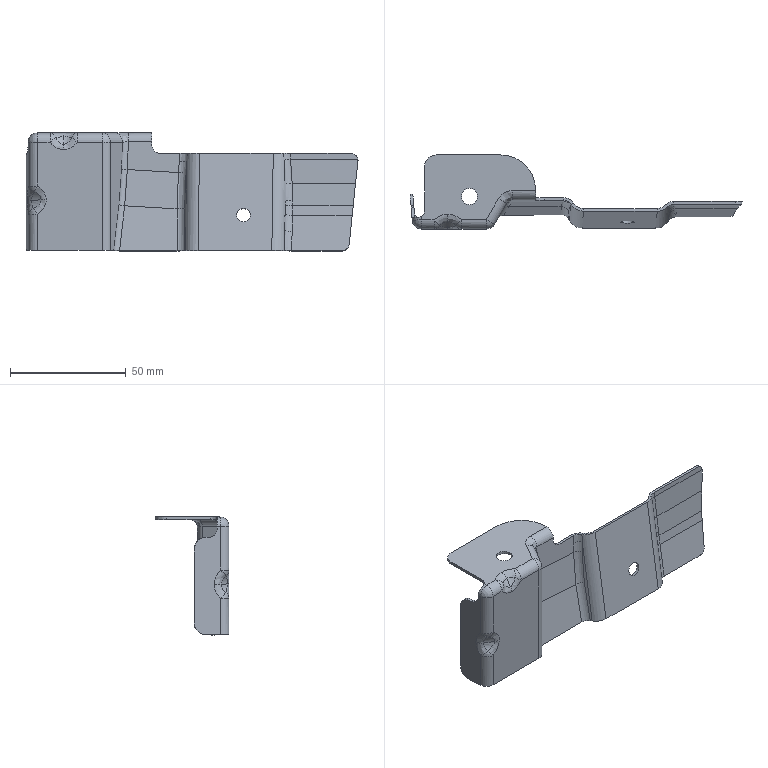Part | 1 solid | 169 faces | box 143.637 x 32 x 51.089 mm | volume 10164 mm3 | spline 74 | cylinder 45 | plane 33 | sphere 12 | other 5 | commonest cylinder face diameters 5.6 x8 8 x8 10 x7 6 x5 7.6 x4 7 x2